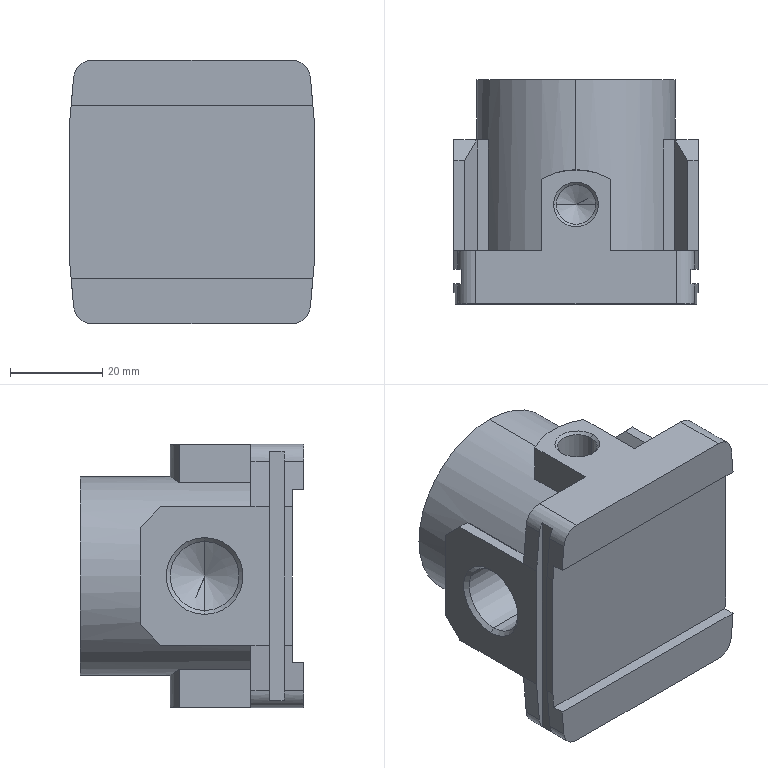Part | SolidWorks | features ICE 8, RefAxis 6, HoleWzd 3, 3DProfileFeature 2, Extrusion 1, RevCut 1, Revolution 1 | 1 solid | 108 faces | box 53 x 48.5 x 57 mm | volume 88299 mm3 | plane 70 | cylinder 24 | cone 14 | commonest cylinder face diameters 8 x4 14.95 x4 36.4 x3 36.8 x3 8.566 x2 8.6 x2